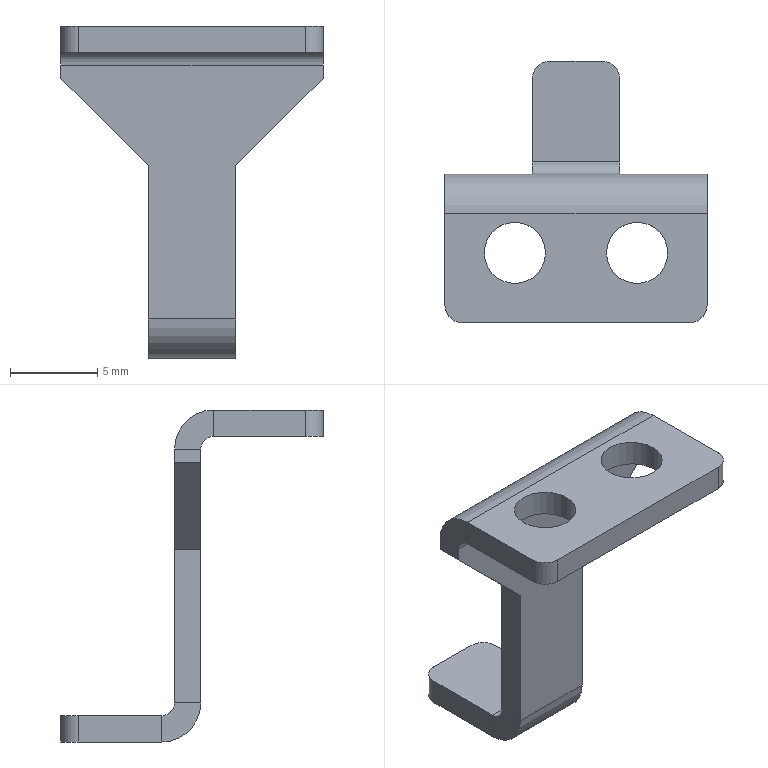Part | STEP file | 06-01-14 photoelectric sensor plate (Default) | 1 solid | 34 faces | box 15 x 15 x 19 mm | volume 381.957 mm3 | plane 22 | cylinder 12 | commonest cylinder face diameters 2 x4 3.5 x4 1.473 x2 4.473 x2
STEP:
#1=CARTESIAN_POINT('',(-5.25,0.5,0.));
#2=VERTEX_POINT('',#1);
#3=CARTESIAN_POINT('',(-1.75,0.5,0.));
#4=VERTEX_POINT('',#3);
#5=CARTESIAN_POINT('',(-3.5,0.5,0.));
#6=DIRECTION('',(0.,0.,1.));
#7=DIRECTION('',(1.,0.,0.));
#8=AXIS2_PLACEMENT_3D('',#5,#6,#7);
#9=CIRCLE('',#8,1.75);
#10=EDGE_CURVE('',#2,#4,#9,.T.);
#11=ORIENTED_EDGE('',*,*,#10,.T.);
#12=CARTESIAN_POINT('',(-1.75,0.5,-1.5));
#13=VERTEX_POINT('',#12);
#14=CARTESIAN_POINT('',(-1.75,0.5,3.5));
#15=DIRECTION('',(0.,0.,-1.));
#16=VECTOR('',#15,1000.);
#17=LINE('',#14,#16);
#18=EDGE_CURVE('',#4,#13,#17,.T.);
#19=ORIENTED_EDGE('',*,*,#18,.T.);
#20=CARTESIAN_POINT('',(-5.25,0.5,-1.5));
#21=VERTEX_POINT('',#20);
#22=CARTESIAN_POINT('',(-3.5,0.5,-1.5));
#23=DIRECTION('',(0.,0.,-1.));
#24=DIRECTION('',(-1.,0.,0.));
#25=AXIS2_PLACEMENT_3D('',#22,#23,#24);
#26=CIRCLE('',#25,1.75);
#27=EDGE_CURVE('',#13,#21,#26,.T.);
#28=ORIENTED_EDGE('',*,*,#27,.T.);
#29=CARTESIAN_POINT('',(-5.25,0.5,3.5));
#30=DIRECTION('',(0.,0.,-1.));
#31=VECTOR('',#30,1000.);
#32=LINE('',#29,#31);
#33=EDGE_CURVE('',#2,#21,#32,.T.);
#34=ORIENTED_EDGE('',*,*,#33,.F.);
#35=EDGE_LOOP('',(#11,#19,#28,#34));
#36=FACE_OUTER_BOUND('',#35,.T.);
#37=CARTESIAN_POINT('',(-3.5,0.5,3.5));
#38=DIRECTION('',(0.,0.,-1.));
#39=DIRECTION('',(-1.,0.,0.));
#40=AXIS2_PLACEMENT_3D('',#37,#38,#39);
#41=CYLINDRICAL_SURFACE('',#40,1.75);
#42=ADVANCED_FACE('',(#36),#41,.F.);
#43=CARTESIAN_POINT('',(1.75,0.5,0.));
#44=VERTEX_POINT('',#43);
#45=CARTESIAN_POINT('',(5.25,0.5,0.));
#46=VERTEX_POINT('',#45);
#47=CARTESIAN_POINT('',(3.5,0.5,0.));
#48=DIRECTION('',(0.,0.,1.));
#49=DIRECTION('',(1.,0.,0.));
#50=AXIS2_PLACEMENT_3D('',#47,#48,#49);
#51=CIRCLE('',#50,1.75);
#52=EDGE_CURVE('',#44,#46,#51,.T.);
#53=ORIENTED_EDGE('',*,*,#52,.T.);
#54=CARTESIAN_POINT('',(5.25,0.5,-1.5));
#55=VERTEX_POINT('',#54);
#56=CARTESIAN_POINT('',(5.25,0.5,3.5));
#57=DIRECTION('',(0.,0.,-1.));
#58=VECTOR('',#57,1000.);
#59=LINE('',#56,#58);
#60=EDGE_CURVE('',#46,#55,#59,.T.);
#61=ORIENTED_EDGE('',*,*,#60,.T.);
#62=CARTESIAN_POINT('',(1.75,0.5,-1.5));
#63=VERTEX_POINT('',#62);
#64=CARTESIAN_POINT('',(3.5,0.5,-1.5));
#65=DIRECTION('',(0.,0.,-1.));
#66=DIRECTION('',(-1.,0.,0.));
#67=AXIS2_PLACEMENT_3D('',#64,#65,#66);
#68=CIRCLE('',#67,1.75);
#69=EDGE_CURVE('',#55,#63,#68,.T.);
#70=ORIENTED_EDGE('',*,*,#69,.T.);
#71=CARTESIAN_POINT('',(1.75,0.5,3.5));
#72=DIRECTION('',(0.,0.,-1.));
#73=VECTOR('',#72,1000.);
#74=LINE('',#71,#73);
#75=EDGE_CURVE('',#44,#63,#74,.T.);
#76=ORIENTED_EDGE('',*,*,#75,.F.);
#77=EDGE_LOOP('',(#53,#61,#70,#76));
#78=FACE_OUTER_BOUND('',#77,.T.);
#79=CARTESIAN_POINT('',(3.5,0.5,3.5));
#80=DIRECTION('',(0.,0.,-1.));
#81=DIRECTION('',(-1.,0.,0.));
#82=AXIS2_PLACEMENT_3D('',#79,#80,#81);
#83=CYLINDRICAL_SURFACE('',#82,1.75);
#84=ADVANCED_FACE('',(#78),#83,.F.);
#85=CARTESIAN_POINT('',(7.5,5.,-3.));
#86=VERTEX_POINT('',#85);
#87=CARTESIAN_POINT('',(7.5,5.,-2.237));
#88=VERTEX_POINT('',#87);
#89=CARTESIAN_POINT('',(7.5,5.,-1.5));
#90=DIRECTION('',(0.,0.,1.));
#91=VECTOR('',#90,1000.);
#92=LINE('',#89,#91);
#93=EDGE_CURVE('',#86,#88,#92,.T.);
#94=ORIENTED_EDGE('',*,*,#93,.F.);
#95=CARTESIAN_POINT('',(2.5,5.,-8.));
#96=VERTEX_POINT('',#95);
#97=CARTESIAN_POINT('',(8.25,5.,-2.25));
#98=DIRECTION('',(0.7071,0.,0.7071));
#99=VECTOR('',#98,1000.);
#100=LINE('',#97,#99);
#101=EDGE_CURVE('',#96,#86,#100,.T.);
#102=ORIENTED_EDGE('',*,*,#101,.F.);
#103=CARTESIAN_POINT('',(2.5,5.,-16.763));
#104=VERTEX_POINT('',#103);
#105=CARTESIAN_POINT('',(2.5,5.,-1.5));
#106=DIRECTION('',(0.,0.,1.));
#107=VECTOR('',#106,1000.);
#108=LINE('',#105,#107);
#109=EDGE_CURVE('',#104,#96,#108,.T.);
#110=ORIENTED_EDGE('',*,*,#109,.F.);
#111=CARTESIAN_POINT('',(-2.5,5.,-16.763));
#112=VERTEX_POINT('',#111);
#113=CARTESIAN_POINT('',(-7.5,5.,-16.763));
#114=DIRECTION('',(1.,0.,0.));
#115=VECTOR('',#114,1000.);
#116=LINE('',#113,#115);
#117=EDGE_CURVE('',#112,#104,#116,.T.);
#118=ORIENTED_EDGE('',*,*,#117,.F.);
#119=CARTESIAN_POINT('',(-2.5,5.,-8.));
#120=VERTEX_POINT('',#119);
#121=CARTESIAN_POINT('',(-2.5,5.,-1.5));
#122=DIRECTION('',(0.,0.,-1.));
#123=VECTOR('',#122,1000.);
#124=LINE('',#121,#123);
#125=EDGE_CURVE('',#120,#112,#124,.T.);
#126=ORIENTED_EDGE('',*,*,#125,.F.);
#127=CARTESIAN_POINT('',(-7.5,5.,-3.));
#128=VERTEX_POINT('',#127);
#129=CARTESIAN_POINT('',(-0.75,5.,-9.75));
#130=DIRECTION('',(0.7071,0.,-0.7071));
#131=VECTOR('',#130,1000.);
#132=LINE('',#129,#131);
#133=EDGE_CURVE('',#128,#120,#132,.T.);
#134=ORIENTED_EDGE('',*,*,#133,.F.);
#135=CARTESIAN_POINT('',(-7.5,5.,-2.237));
#136=VERTEX_POINT('',#135);
#137=CARTESIAN_POINT('',(-7.5,5.,-17.5));
#138=DIRECTION('',(0.,0.,-1.));
#139=VECTOR('',#138,1000.);
#140=LINE('',#137,#139);
#141=EDGE_CURVE('',#136,#128,#140,.T.);
#142=ORIENTED_EDGE('',*,*,#141,.F.);
#143=CARTESIAN_POINT('',(7.5,5.,-2.237));
#144=DIRECTION('',(1.,0.,0.));
#145=VECTOR('',#144,1000.);
#146=LINE('',#143,#145);
#147=EDGE_CURVE('',#136,#88,#146,.T.);
#148=ORIENTED_EDGE('',*,*,#147,.T.);
#149=EDGE_LOOP('',(#94,#102,#110,#118,#126,#134,#142,#148));
#150=FACE_OUTER_BOUND('',#149,.T.);
#151=CARTESIAN_POINT('',(7.5,5.,-1.5));
#152=DIRECTION('',(0.,1.,0.));
#153=DIRECTION('',(0.,0.,1.));
#154=AXIS2_PLACEMENT_3D('',#151,#152,#153);
#155=PLANE('',#154);
#156=ADVANCED_FACE('',(#150),#155,.T.);
#157=CARTESIAN_POINT('',(2.5,3.5,-8.));
#158=VERTEX_POINT('',#157);
#159=CARTESIAN_POINT('',(7.5,3.5,-3.));
#160=VERTEX_POINT('',#159);
#161=CARTESIAN_POINT('',(8.25,3.5,-2.25));
#162=DIRECTION('',(0.7071,0.,0.7071));
#163=VECTOR('',#162,1000.);
#164=LINE('',#161,#163);
#165=EDGE_CURVE('',#158,#160,#164,.T.);
#166=ORIENTED_EDGE('',*,*,#165,.T.);
#167=CARTESIAN_POINT('',(7.5,3.5,-2.237));
#168=VERTEX_POINT('',#167);
#169=CARTESIAN_POINT('',(7.5,3.5,-1.5));
#170=DIRECTION('',(0.,0.,1.));
#171=VECTOR('',#170,1000.);
#172=LINE('',#169,#171);
#173=EDGE_CURVE('',#160,#168,#172,.T.);
#174=ORIENTED_EDGE('',*,*,#173,.T.);
#175=CARTESIAN_POINT('',(-7.5,3.5,-2.237));
#176=VERTEX_POINT('',#175);
#177=CARTESIAN_POINT('',(-7.5,3.5,-2.237));
#178=DIRECTION('',(1.,0.,0.));
#179=VECTOR('',#178,1000.);
#180=LINE('',#177,#179);
#181=EDGE_CURVE('',#176,#168,#180,.T.);
#182=ORIENTED_EDGE('',*,*,#181,.F.);
#183=CARTESIAN_POINT('',(-7.5,3.5,-3.));
#184=VERTEX_POINT('',#183);
#185=CARTESIAN_POINT('',(-7.5,3.5,-17.5));
#186=DIRECTION('',(0.,0.,-1.));
#187=VECTOR('',#186,1000.);
#188=LINE('',#185,#187);
#189=EDGE_CURVE('',#176,#184,#188,.T.);
#190=ORIENTED_EDGE('',*,*,#189,.T.);
#191=CARTESIAN_POINT('',(-2.5,3.5,-8.));
#192=VERTEX_POINT('',#191);
#193=CARTESIAN_POINT('',(-0.75,3.5,-9.75));
#194=DIRECTION('',(0.7071,0.,-0.7071));
#195=VECTOR('',#194,1000.);
#196=LINE('',#193,#195);
#197=EDGE_CURVE('',#184,#192,#196,.T.);
#198=ORIENTED_EDGE('',*,*,#197,.T.);
#199=CARTESIAN_POINT('',(-2.5,3.5,-16.763));
#200=VERTEX_POINT('',#199);
#201=CARTESIAN_POINT('',(-2.5,3.5,-1.5));
#202=DIRECTION('',(0.,0.,-1.));
#203=VECTOR('',#202,1000.);
#204=LINE('',#201,#203);
#205=EDGE_CURVE('',#192,#200,#204,.T.);
#206=ORIENTED_EDGE('',*,*,#205,.T.);
#207=CARTESIAN_POINT('',(2.5,3.5,-16.763));
#208=VERTEX_POINT('',#207);
#209=CARTESIAN_POINT('',(-7.5,3.5,-16.763));
#210=DIRECTION('',(1.,0.,0.));
#211=VECTOR('',#210,1000.);
#212=LINE('',#209,#211);
#213=EDGE_CURVE('',#200,#208,#212,.T.);
#214=ORIENTED_EDGE('',*,*,#213,.T.);
#215=CARTESIAN_POINT('',(2.5,3.5,-1.5));
#216=DIRECTION('',(0.,0.,1.));
#217=VECTOR('',#216,1000.);
#218=LINE('',#215,#217);
#219=EDGE_CURVE('',#208,#158,#218,.T.);
#220=ORIENTED_EDGE('',*,*,#219,.T.);
#221=EDGE_LOOP('',(#166,#174,#182,#190,#198,#206,#214,#220));
#222=FACE_OUTER_BOUND('',#221,.T.);
#223=CARTESIAN_POINT('',(7.5,3.5,-1.5));
#224=DIRECTION('',(0.,1.,0.));
#225=DIRECTION('',(0.,0.,1.));
#226=AXIS2_PLACEMENT_3D('',#223,#224,#225);
#227=PLANE('',#226);
#228=ADVANCED_FACE('',(#222),#227,.F.);
#229=CARTESIAN_POINT('',(2.5,5.737,-19.));
#230=VERTEX_POINT('',#229);
#231=CARTESIAN_POINT('',(-2.5,5.737,-19.));
#232=VERTEX_POINT('',#231);
#233=CARTESIAN_POINT('',(-7.5,5.737,-19.));
#234=DIRECTION('',(-1.,0.,0.));
#235=VECTOR('',#234,1000.);
#236=LINE('',#233,#235);
#237=EDGE_CURVE('',#230,#232,#236,.T.);
#238=ORIENTED_EDGE('',*,*,#237,.F.);
#239=CARTESIAN_POINT('',(2.5,5.737,-16.763));
#240=DIRECTION('',(1.,0.,0.));
#241=DIRECTION('',(0.,0.,1.));
#242=AXIS2_PLACEMENT_3D('',#239,#240,#241);
#243=CIRCLE('',#242,2.237);
#244=EDGE_CURVE('',#208,#230,#243,.T.);
#245=ORIENTED_EDGE('',*,*,#244,.F.);
#246=ORIENTED_EDGE('',*,*,#213,.F.);
#247=CARTESIAN_POINT('',(-2.5,5.737,-16.763));
#248=DIRECTION('',(-1.,0.,0.));
#249=DIRECTION('',(0.,0.,-1.));
#250=AXIS2_PLACEMENT_3D('',#247,#248,#249);
#251=CIRCLE('',#250,2.237);
#252=EDGE_CURVE('',#232,#200,#251,.T.);
#253=ORIENTED_EDGE('',*,*,#252,.F.);
#254=EDGE_LOOP('',(#238,#245,#246,#253));
#255=FACE_OUTER_BOUND('',#254,.T.);
#256=CARTESIAN_POINT('',(-7.5,5.737,-16.763));
#257=DIRECTION('',(-1.,0.,0.));
#258=DIRECTION('',(0.,0.,-1.));
#259=AXIS2_PLACEMENT_3D('',#256,#257,#258);
#260=CYLINDRICAL_SURFACE('',#259,2.237);
#261=ADVANCED_FACE('',(#255),#260,.T.);
#262=CARTESIAN_POINT('',(2.5,5.737,-17.5));
#263=VERTEX_POINT('',#262);
#264=CARTESIAN_POINT('',(2.5,5.737,-16.763));
#265=DIRECTION('',(1.,0.,0.));
#266=DIRECTION('',(0.,0.,1.));
#267=AXIS2_PLACEMENT_3D('',#264,#265,#266);
#268=CIRCLE('',#267,0.7366);
#269=EDGE_CURVE('',#104,#263,#268,.T.);
#270=ORIENTED_EDGE('',*,*,#269,.T.);
#271=CARTESIAN_POINT('',(-2.5,5.737,-17.5));
#272=VERTEX_POINT('',#271);
#273=CARTESIAN_POINT('',(7.5,5.737,-17.5));
#274=DIRECTION('',(-1.,0.,0.));
#275=VECTOR('',#274,1000.);
#276=LINE('',#273,#275);
#277=EDGE_CURVE('',#263,#272,#276,.T.);
#278=ORIENTED_EDGE('',*,*,#277,.T.);
#279=CARTESIAN_POINT('',(-2.5,5.737,-16.763));
#280=DIRECTION('',(-1.,0.,0.));
#281=DIRECTION('',(0.,0.,1.));
#282=AXIS2_PLACEMENT_3D('',#279,#280,#281);
#283=CIRCLE('',#282,0.7366);
#284=EDGE_CURVE('',#272,#112,#283,.T.);
#285=ORIENTED_EDGE('',*,*,#284,.T.);
#286=ORIENTED_EDGE('',*,*,#117,.T.);
#287=EDGE_LOOP('',(#270,#278,#285,#286));
#288=FACE_OUTER_BOUND('',#287,.T.);
#289=CARTESIAN_POINT('',(-7.5,5.737,-16.763));
#290=DIRECTION('',(-1.,0.,0.));
#291=DIRECTION('',(0.,0.,-1.));
#292=AXIS2_PLACEMENT_3D('',#289,#290,#291);
#293=CYLINDRICAL_SURFACE('',#292,0.7366);
#294=ADVANCED_FACE('',(#288),#293,.F.);
#295=CARTESIAN_POINT('',(1.5,11.5,-19.));
#296=VERTEX_POINT('',#295);
#297=CARTESIAN_POINT('',(-1.5,11.5,-19.));
#298=VERTEX_POINT('',#297);
#299=CARTESIAN_POINT('',(-7.5,11.5,-19.));
#300=DIRECTION('',(-1.,0.,0.));
#301=VECTOR('',#300,1000.);
#302=LINE('',#299,#301);
#303=EDGE_CURVE('',#296,#298,#302,.T.);
#304=ORIENTED_EDGE('',*,*,#303,.F.);
#305=CARTESIAN_POINT('',(2.5,10.5,-19.));
#306=VERTEX_POINT('',#305);
#307=CARTESIAN_POINT('',(1.5,10.5,-19.));
#308=DIRECTION('',(0.,0.,-1.));
#309=DIRECTION('',(-1.,0.,0.));
#310=AXIS2_PLACEMENT_3D('',#307,#308,#309);
#311=CIRCLE('',#310,1.);
#312=EDGE_CURVE('',#296,#306,#311,.T.);
#313=ORIENTED_EDGE('',*,*,#312,.T.);
#314=CARTESIAN_POINT('',(2.5,5.,-19.));
#315=DIRECTION('',(0.,1.,0.));
#316=VECTOR('',#315,1000.);
#317=LINE('',#314,#316);
#318=EDGE_CURVE('',#230,#306,#317,.T.);
#319=ORIENTED_EDGE('',*,*,#318,.F.);
#320=ORIENTED_EDGE('',*,*,#237,.T.);
#321=CARTESIAN_POINT('',(-2.5,10.5,-19.));
#322=VERTEX_POINT('',#321);
#323=CARTESIAN_POINT('',(-2.5,5.,-19.));
#324=DIRECTION('',(0.,-1.,0.));
#325=VECTOR('',#324,1000.);
#326=LINE('',#323,#325);
#327=EDGE_CURVE('',#322,#232,#326,.T.);
#328=ORIENTED_EDGE('',*,*,#327,.F.);
#329=CARTESIAN_POINT('',(-1.5,10.5,-19.));
#330=DIRECTION('',(0.,0.,-1.));
#331=DIRECTION('',(-1.,0.,0.));
#332=AXIS2_PLACEMENT_3D('',#329,#330,#331);
#333=CIRCLE('',#332,1.);
#334=EDGE_CURVE('',#322,#298,#333,.T.);
#335=ORIENTED_EDGE('',*,*,#334,.T.);
#336=EDGE_LOOP('',(#304,#313,#319,#320,#328,#335));
#337=FACE_OUTER_BOUND('',#336,.T.);
#338=CARTESIAN_POINT('',(-7.5,5.,-19.));
#339=DIRECTION('',(0.,0.,-1.));
#340=DIRECTION('',(-1.,0.,0.));
#341=AXIS2_PLACEMENT_3D('',#338,#339,#340);
#342=PLANE('',#341);
#343=ADVANCED_FACE('',(#337),#342,.T.);
#344=CARTESIAN_POINT('',(2.5,10.5,-17.5));
#345=VERTEX_POINT('',#344);
#346=CARTESIAN_POINT('',(2.5,5.,-17.5));
#347=DIRECTION('',(0.,1.,0.));
#348=VECTOR('',#347,1000.);
#349=LINE('',#346,#348);
#350=EDGE_CURVE('',#263,#345,#349,.T.);
#351=ORIENTED_EDGE('',*,*,#350,.T.);
#352=CARTESIAN_POINT('',(1.5,11.5,-17.5));
#353=VERTEX_POINT('',#352);
#354=CARTESIAN_POINT('',(1.5,10.5,-17.5));
#355=DIRECTION('',(0.,0.,1.));
#356=DIRECTION('',(-1.,0.,0.));
#357=AXIS2_PLACEMENT_3D('',#354,#355,#356);
#358=CIRCLE('',#357,1.);
#359=EDGE_CURVE('',#345,#353,#358,.T.);
#360=ORIENTED_EDGE('',*,*,#359,.T.);
#361=CARTESIAN_POINT('',(-1.5,11.5,-17.5));
#362=VERTEX_POINT('',#361);
#363=CARTESIAN_POINT('',(-7.5,11.5,-17.5));
#364=DIRECTION('',(-1.,0.,0.));
#365=VECTOR('',#364,1000.);
#366=LINE('',#363,#365);
#367=EDGE_CURVE('',#353,#362,#366,.T.);
#368=ORIENTED_EDGE('',*,*,#367,.T.);
#369=CARTESIAN_POINT('',(-2.5,10.5,-17.5));
#370=VERTEX_POINT('',#369);
#371=CARTESIAN_POINT('',(-1.5,10.5,-17.5));
#372=DIRECTION('',(0.,0.,1.));
#373=DIRECTION('',(-1.,0.,0.));
#374=AXIS2_PLACEMENT_3D('',#371,#372,#373);
#375=CIRCLE('',#374,1.);
#376=EDGE_CURVE('',#362,#370,#375,.T.);
#377=ORIENTED_EDGE('',*,*,#376,.T.);
#378=CARTESIAN_POINT('',(-2.5,5.,-17.5));
#379=DIRECTION('',(0.,-1.,0.));
#380=VECTOR('',#379,1000.);
#381=LINE('',#378,#380);
#382=EDGE_CURVE('',#370,#272,#381,.T.);
#383=ORIENTED_EDGE('',*,*,#382,.T.);
#384=ORIENTED_EDGE('',*,*,#277,.F.);
#385=EDGE_LOOP('',(#351,#360,#368,#377,#383,#384));
#386=FACE_OUTER_BOUND('',#385,.T.);
#387=CARTESIAN_POINT('',(-7.5,5.,-17.5));
#388=DIRECTION('',(0.,0.,-1.));
#389=DIRECTION('',(-1.,0.,0.));
#390=AXIS2_PLACEMENT_3D('',#387,#388,#389);
#391=PLANE('',#390);
#392=ADVANCED_FACE('',(#386),#391,.F.);
#393=ORIENTED_EDGE('',*,*,#367,.F.);
#394=CARTESIAN_POINT('',(1.5,11.5,-19.));
#395=DIRECTION('',(0.,0.,-1.));
#396=VECTOR('',#395,1000.);
#397=LINE('',#394,#396);
#398=EDGE_CURVE('',#353,#296,#397,.T.);
#399=ORIENTED_EDGE('',*,*,#398,.T.);
#400=ORIENTED_EDGE('',*,*,#303,.T.);
#401=CARTESIAN_POINT('',(-1.5,11.5,-19.));
#402=DIRECTION('',(0.,0.,1.));
#403=VECTOR('',#402,1000.);
#404=LINE('',#401,#403);
#405=EDGE_CURVE('',#298,#362,#404,.T.);
#406=ORIENTED_EDGE('',*,*,#405,.T.);
#407=EDGE_LOOP('',(#393,#399,#400,#406));
#408=FACE_OUTER_BOUND('',#407,.T.);
#409=CARTESIAN_POINT('',(-7.5,11.5,-19.));
#410=DIRECTION('',(0.,1.,0.));
#411=DIRECTION('',(0.,0.,1.));
#412=AXIS2_PLACEMENT_3D('',#409,#410,#411);
#413=PLANE('',#412);
#414=ADVANCED_FACE('',(#408),#413,.T.);
#415=ORIENTED_EDGE('',*,*,#173,.F.);
#416=CARTESIAN_POINT('',(7.5,5.,-3.));
#417=DIRECTION('',(0.,-1.,0.));
#418=VECTOR('',#417,1000.);
#419=LINE('',#416,#418);
#420=EDGE_CURVE('',#86,#160,#419,.T.);
#421=ORIENTED_EDGE('',*,*,#420,.F.);
#422=ORIENTED_EDGE('',*,*,#93,.T.);
#423=CARTESIAN_POINT('',(7.5,3.5,-2.237));
#424=DIRECTION('',(0.,1.,0.));
#425=VECTOR('',#424,1000.);
#426=LINE('',#423,#425);
#427=EDGE_CURVE('',#168,#88,#426,.T.);
#428=ORIENTED_EDGE('',*,*,#427,.F.);
#429=EDGE_LOOP('',(#415,#421,#422,#428));
#430=FACE_OUTER_BOUND('',#429,.T.);
#431=CARTESIAN_POINT('',(7.5,5.,-1.5));
#432=DIRECTION('',(1.,0.,0.));
#433=DIRECTION('',(0.,0.,-1.));
#434=AXIS2_PLACEMENT_3D('',#431,#432,#433);
#435=PLANE('',#434);
#436=ADVANCED_FACE('',(#430),#435,.T.);
#437=ORIENTED_EDGE('',*,*,#141,.T.);
#438=CARTESIAN_POINT('',(-7.5,5.,-3.));
#439=DIRECTION('',(0.,-1.,0.));
#440=VECTOR('',#439,1000.);
#441=LINE('',#438,#440);
#442=EDGE_CURVE('',#128,#184,#441,.T.);
#443=ORIENTED_EDGE('',*,*,#442,.T.);
#444=ORIENTED_EDGE('',*,*,#189,.F.);
#445=CARTESIAN_POINT('',(-7.5,3.5,-2.237));
#446=DIRECTION('',(0.,1.,0.));
#447=VECTOR('',#446,1000.);
#448=LINE('',#445,#447);
#449=EDGE_CURVE('',#176,#136,#448,.T.);
#450=ORIENTED_EDGE('',*,*,#449,.T.);
#451=EDGE_LOOP('',(#437,#443,#444,#450));
#452=FACE_OUTER_BOUND('',#451,.T.);
#453=CARTESIAN_POINT('',(-7.5,5.,-17.5));
#454=DIRECTION('',(-1.,0.,0.));
#455=DIRECTION('',(0.,0.,1.));
#456=AXIS2_PLACEMENT_3D('',#453,#454,#455);
#457=PLANE('',#456);
#458=ADVANCED_FACE('',(#452),#457,.T.);
#459=CARTESIAN_POINT('',(7.5,-2.5,0.));
#460=VERTEX_POINT('',#459);
#461=CARTESIAN_POINT('',(7.5,2.763,0.));
#462=VERTEX_POINT('',#461);
#463=CARTESIAN_POINT('',(7.5,3.5,0.));
#464=DIRECTION('',(0.,1.,0.));
#465=VECTOR('',#464,1000.);
#466=LINE('',#463,#465);
#467=EDGE_CURVE('',#460,#462,#466,.T.);
#468=ORIENTED_EDGE('',*,*,#467,.F.);
#469=CARTESIAN_POINT('',(7.5,-2.5,-1.5));
#470=VERTEX_POINT('',#469);
#471=CARTESIAN_POINT('',(7.5,-2.5,-1.5));
#472=DIRECTION('',(0.,0.,-1.));
#473=VECTOR('',#472,1000.);
#474=LINE('',#471,#473);
#475=EDGE_CURVE('',#460,#470,#474,.T.);
#476=ORIENTED_EDGE('',*,*,#475,.T.);
#477=CARTESIAN_POINT('',(7.5,2.763,-1.5));
#478=VERTEX_POINT('',#477);
#479=CARTESIAN_POINT('',(7.5,3.5,-1.5));
#480=DIRECTION('',(0.,1.,0.));
#481=VECTOR('',#480,1000.);
#482=LINE('',#479,#481);
#483=EDGE_CURVE('',#470,#478,#482,.T.);
#484=ORIENTED_EDGE('',*,*,#483,.T.);
#485=CARTESIAN_POINT('',(7.5,2.763,-1.5));
#486=DIRECTION('',(0.,0.,1.));
#487=VECTOR('',#486,1000.);
#488=LINE('',#485,#487);
#489=EDGE_CURVE('',#478,#462,#488,.T.);
#490=ORIENTED_EDGE('',*,*,#489,.T.);
#491=EDGE_LOOP('',(#468,#476,#484,#490));
#492=FACE_OUTER_BOUND('',#491,.T.);
#493=CARTESIAN_POINT('',(7.5,3.5,-1.5));
#494=DIRECTION('',(1.,0.,0.));
#495=DIRECTION('',(0.,1.,0.));
#496=AXIS2_PLACEMENT_3D('',#493,#494,#495);
#497=PLANE('',#496);
#498=ADVANCED_FACE('',(#492),#497,.T.);
#499=CARTESIAN_POINT('',(-3.5,0.5,-1.5));
#500=DIRECTION('',(0.,0.,-1.));
#501=DIRECTION('',(-1.,0.,0.));
#502=AXIS2_PLACEMENT_3D('',#499,#500,#501);
#503=CIRCLE('',#502,1.75);
#504=EDGE_CURVE('',#21,#13,#503,.T.);
#505=ORIENTED_EDGE('',*,*,#504,.F.);
#506=ORIENTED_EDGE('',*,*,#27,.F.);
#507=EDGE_LOOP('',(#505,#506));
#508=FACE_BOUND('',#507,.T.);
#509=CARTESIAN_POINT('',(3.5,0.5,-1.5));
#510=DIRECTION('',(0.,0.,-1.));
#511=DIRECTION('',(-1.,0.,0.));
#512=AXIS2_PLACEMENT_3D('',#509,#510,#511);
#513=CIRCLE('',#512,1.75);
#514=EDGE_CURVE('',#63,#55,#513,.T.);
#515=ORIENTED_EDGE('',*,*,#514,.F.);
#516=ORIENTED_EDGE('',*,*,#69,.F.);
#517=EDGE_LOOP('',(#515,#516));
#518=FACE_BOUND('',#517,.T.);
#519=ORIENTED_EDGE('',*,*,#483,.F.);
#520=CARTESIAN_POINT('',(6.5,-3.5,-1.5));
#521=VERTEX_POINT('',#520);
#522=CARTESIAN_POINT('',(6.5,-2.5,-1.5));
#523=DIRECTION('',(0.,0.,-1.));
#524=DIRECTION('',(1.,0.,0.));
#525=AXIS2_PLACEMENT_3D('',#522,#523,#524);
#526=CIRCLE('',#525,1.);
#527=EDGE_CURVE('',#470,#521,#526,.T.);
#528=ORIENTED_EDGE('',*,*,#527,.T.);
#529=CARTESIAN_POINT('',(-6.5,-3.5,-1.5));
#530=VERTEX_POINT('',#529);
#531=CARTESIAN_POINT('',(-7.5,-3.5,-1.5));
#532=DIRECTION('',(1.,0.,0.));
#533=VECTOR('',#532,1000.);
#534=LINE('',#531,#533);
#535=EDGE_CURVE('',#530,#521,#534,.T.);
#536=ORIENTED_EDGE('',*,*,#535,.F.);
#537=CARTESIAN_POINT('',(-7.5,-2.5,-1.5));
#538=VERTEX_POINT('',#537);
#539=CARTESIAN_POINT('',(-6.5,-2.5,-1.5));
#540=DIRECTION('',(0.,0.,-1.));
#541=DIRECTION('',(1.,0.,0.));
#542=AXIS2_PLACEMENT_3D('',#539,#540,#541);
#543=CIRCLE('',#542,1.);
#544=EDGE_CURVE('',#530,#538,#543,.T.);
#545=ORIENTED_EDGE('',*,*,#544,.T.);
#546=CARTESIAN_POINT('',(-7.5,2.763,-1.5));
#547=VERTEX_POINT('',#546);
#548=CARTESIAN_POINT('',(-7.5,3.5,-1.5));
#549=DIRECTION('',(0.,-1.,0.));
#550=VECTOR('',#549,1000.);
#551=LINE('',#548,#550);
#552=EDGE_CURVE('',#547,#538,#551,.T.);
#553=ORIENTED_EDGE('',*,*,#552,.F.);
#554=CARTESIAN_POINT('',(7.5,2.763,-1.5));
#555=DIRECTION('',(-1.,0.,0.));
#556=VECTOR('',#555,1000.);
#557=LINE('',#554,#556);
#558=EDGE_CURVE('',#478,#547,#557,.T.);
#559=ORIENTED_EDGE('',*,*,#558,.F.);
#560=EDGE_LOOP('',(#519,#528,#536,#545,#553,#559));
#561=FACE_OUTER_BOUND('',#560,.T.);
#562=CARTESIAN_POINT('',(7.5,-3.5,-1.5));
#563=DIRECTION('',(0.,0.,1.));
#564=DIRECTION('',(1.,0.,0.));
#565=AXIS2_PLACEMENT_3D('',#562,#563,#564);
#566=PLANE('',#565);
#567=ADVANCED_FACE('',(#508,#518,#561),#566,.F.);
#568=ORIENTED_EDGE('',*,*,#10,.F.);
#569=CARTESIAN_POINT('',(-3.5,0.5,0.));
#570=DIRECTION('',(0.,0.,1.));
#571=DIRECTION('',(1.,0.,0.));
#572=AXIS2_PLACEMENT_3D('',#569,#570,#571);
#573=CIRCLE('',#572,1.75);
#574=EDGE_CURVE('',#4,#2,#573,.T.);
#575=ORIENTED_EDGE('',*,*,#574,.F.);
#576=EDGE_LOOP('',(#568,#575));
#577=FACE_BOUND('',#576,.T.);
#578=ORIENTED_EDGE('',*,*,#52,.F.);
#579=CARTESIAN_POINT('',(3.5,0.5,0.));
#580=DIRECTION('',(0.,0.,1.));
#581=DIRECTION('',(1.,0.,0.));
#582=AXIS2_PLACEMENT_3D('',#579,#580,#581);
#583=CIRCLE('',#582,1.75);
#584=EDGE_CURVE('',#46,#44,#583,.T.);
#585=ORIENTED_EDGE('',*,*,#584,.F.);
#586=EDGE_LOOP('',(#578,#585));
#587=FACE_BOUND('',#586,.T.);
#588=CARTESIAN_POINT('',(-6.5,-3.5,0.));
#589=VERTEX_POINT('',#588);
#590=CARTESIAN_POINT('',(6.5,-3.5,0.));
#591=VERTEX_POINT('',#590);
#592=CARTESIAN_POINT('',(-7.5,-3.5,0.));
#593=DIRECTION('',(1.,0.,0.));
#594=VECTOR('',#593,1000.);
#595=LINE('',#592,#594);
#596=EDGE_CURVE('',#589,#591,#595,.T.);
#597=ORIENTED_EDGE('',*,*,#596,.T.);
#598=CARTESIAN_POINT('',(6.5,-2.5,0.));
#599=DIRECTION('',(0.,0.,1.));
#600=DIRECTION('',(1.,0.,0.));
#601=AXIS2_PLACEMENT_3D('',#598,#599,#600);
#602=CIRCLE('',#601,1.);
#603=EDGE_CURVE('',#591,#460,#602,.T.);
#604=ORIENTED_EDGE('',*,*,#603,.T.);
#605=ORIENTED_EDGE('',*,*,#467,.T.);
#606=CARTESIAN_POINT('',(-7.5,2.763,0.));
#607=VERTEX_POINT('',#606);
#608=CARTESIAN_POINT('',(7.5,2.763,0.));
#609=DIRECTION('',(-1.,0.,0.));
#610=VECTOR('',#609,1000.);
#611=LINE('',#608,#610);
#612=EDGE_CURVE('',#462,#607,#611,.T.);
#613=ORIENTED_EDGE('',*,*,#612,.T.);
#614=CARTESIAN_POINT('',(-7.5,-2.5,0.));
#615=VERTEX_POINT('',#614);
#616=CARTESIAN_POINT('',(-7.5,3.5,0.));
#617=DIRECTION('',(0.,-1.,0.));
#618=VECTOR('',#617,1000.);
#619=LINE('',#616,#618);
#620=EDGE_CURVE('',#607,#615,#619,.T.);
#621=ORIENTED_EDGE('',*,*,#620,.T.);
#622=CARTESIAN_POINT('',(-6.5,-2.5,0.));
#623=DIRECTION('',(0.,0.,1.));
#624=DIRECTION('',(1.,0.,0.));
#625=AXIS2_PLACEMENT_3D('',#622,#623,#624);
#626=CIRCLE('',#625,1.);
#627=EDGE_CURVE('',#615,#589,#626,.T.);
#628=ORIENTED_EDGE('',*,*,#627,.T.);
#629=EDGE_LOOP('',(#597,#604,#605,#613,#621,#628));
#630=FACE_OUTER_BOUND('',#629,.T.);
#631=CARTESIAN_POINT('',(7.5,-3.5,0.));
#632=DIRECTION('',(0.,0.,1.));
#633=DIRECTION('',(1.,0.,0.));
#634=AXIS2_PLACEMENT_3D('',#631,#632,#633);
#635=PLANE('',#634);
#636=ADVANCED_FACE('',(#577,#587,#630),#635,.T.);
#637=ORIENTED_EDGE('',*,*,#535,.T.);
#638=CARTESIAN_POINT('',(6.5,-3.5,-1.5));
#639=DIRECTION('',(0.,0.,1.));
#640=VECTOR('',#639,1000.);
#641=LINE('',#638,#640);
#642=EDGE_CURVE('',#521,#591,#641,.T.);
#643=ORIENTED_EDGE('',*,*,#642,.T.);
#644=ORIENTED_EDGE('',*,*,#596,.F.);
#645=CARTESIAN_POINT('',(-6.5,-3.5,-1.5));
#646=DIRECTION('',(0.,0.,-1.));
#647=VECTOR('',#646,1000.);
#648=LINE('',#645,#647);
#649=EDGE_CURVE('',#589,#530,#648,.T.);
#650=ORIENTED_EDGE('',*,*,#649,.T.);
#651=EDGE_LOOP('',(#637,#643,#644,#650));
#652=FACE_OUTER_BOUND('',#651,.T.);
#653=CARTESIAN_POINT('',(-7.5,-3.5,-1.5));
#654=DIRECTION('',(0.,-1.,0.));
#655=DIRECTION('',(0.,0.,-1.));
#656=AXIS2_PLACEMENT_3D('',#653,#654,#655);
#657=PLANE('',#656);
#658=ADVANCED_FACE('',(#652),#657,.T.);
#659=ORIENTED_EDGE('',*,*,#552,.T.);
#660=CARTESIAN_POINT('',(-7.5,-2.5,-1.5));
#661=DIRECTION('',(0.,0.,1.));
#662=VECTOR('',#661,1000.);
#663=LINE('',#660,#662);
#664=EDGE_CURVE('',#538,#615,#663,.T.);
#665=ORIENTED_EDGE('',*,*,#664,.T.);
#666=ORIENTED_EDGE('',*,*,#620,.F.);
#667=CARTESIAN_POINT('',(-7.5,2.763,-1.5));
#668=DIRECTION('',(0.,0.,1.));
#669=VECTOR('',#668,1000.);
#670=LINE('',#667,#669);
#671=EDGE_CURVE('',#547,#607,#670,.T.);
#672=ORIENTED_EDGE('',*,*,#671,.F.);
#673=EDGE_LOOP('',(#659,#665,#666,#672));
#674=FACE_OUTER_BOUND('',#673,.T.);
#675=CARTESIAN_POINT('',(-7.5,3.5,-1.5));
#676=DIRECTION('',(-1.,0.,0.));
#677=DIRECTION('',(0.,-1.,0.));
#678=AXIS2_PLACEMENT_3D('',#675,#676,#677);
#679=PLANE('',#678);
#680=ADVANCED_FACE('',(#674),#679,.T.);
#681=ORIENTED_EDGE('',*,*,#449,.F.);
#682=CARTESIAN_POINT('',(-7.5,2.763,-2.237));
#683=DIRECTION('',(-1.,0.,0.));
#684=DIRECTION('',(0.,0.,-1.));
#685=AXIS2_PLACEMENT_3D('',#682,#683,#684);
#686=CIRCLE('',#685,0.7366);
#687=EDGE_CURVE('',#547,#176,#686,.T.);
#688=ORIENTED_EDGE('',*,*,#687,.F.);
#689=ORIENTED_EDGE('',*,*,#671,.T.);
#690=CARTESIAN_POINT('',(-7.5,2.763,-2.237));
#691=DIRECTION('',(-1.,0.,0.));
#692=DIRECTION('',(0.,0.,-1.));
#693=AXIS2_PLACEMENT_3D('',#690,#691,#692);
#694=CIRCLE('',#693,2.237);
#695=EDGE_CURVE('',#607,#136,#694,.T.);
#696=ORIENTED_EDGE('',*,*,#695,.T.);
#697=EDGE_LOOP('',(#681,#688,#689,#696));
#698=FACE_OUTER_BOUND('',#697,.T.);
#699=CARTESIAN_POINT('',(-7.5,2.763,-2.237));
#700=DIRECTION('',(-1.,0.,0.));
#701=DIRECTION('',(0.,0.,1.));
#702=AXIS2_PLACEMENT_3D('',#699,#700,#701);
#703=PLANE('',#702);
#704=ADVANCED_FACE('',(#698),#703,.T.);
#705=CARTESIAN_POINT('',(7.5,2.763,-2.237));
#706=DIRECTION('',(1.,0.,0.));
#707=DIRECTION('',(0.,0.,-1.));
#708=AXIS2_PLACEMENT_3D('',#705,#706,#707);
#709=CIRCLE('',#708,0.7366);
#710=EDGE_CURVE('',#168,#478,#709,.T.);
#711=ORIENTED_EDGE('',*,*,#710,.F.);
#712=ORIENTED_EDGE('',*,*,#427,.T.);
#713=CARTESIAN_POINT('',(7.5,2.763,-2.237));
#714=DIRECTION('',(1.,0.,0.));
#715=DIRECTION('',(0.,0.,-1.));
#716=AXIS2_PLACEMENT_3D('',#713,#714,#715);
#717=CIRCLE('',#716,2.237);
#718=EDGE_CURVE('',#88,#462,#717,.T.);
#719=ORIENTED_EDGE('',*,*,#718,.T.);
#720=ORIENTED_EDGE('',*,*,#489,.F.);
#721=EDGE_LOOP('',(#711,#712,#719,#720));
#722=FACE_OUTER_BOUND('',#721,.T.);
#723=CARTESIAN_POINT('',(7.5,2.763,-2.237));
#724=DIRECTION('',(-1.,0.,0.));
#725=DIRECTION('',(0.,0.,1.));
#726=AXIS2_PLACEMENT_3D('',#723,#724,#725);
#727=PLANE('',#726);
#728=ADVANCED_FACE('',(#722),#727,.F.);
#729=ORIENTED_EDGE('',*,*,#612,.F.);
#730=ORIENTED_EDGE('',*,*,#718,.F.);
#731=ORIENTED_EDGE('',*,*,#147,.F.);
#732=ORIENTED_EDGE('',*,*,#695,.F.);
#733=EDGE_LOOP('',(#729,#730,#731,#732));
#734=FACE_OUTER_BOUND('',#733,.T.);
#735=CARTESIAN_POINT('',(7.5,2.763,-2.237));
#736=DIRECTION('',(1.,0.,0.));
#737=DIRECTION('',(0.,1.,0.));
#738=AXIS2_PLACEMENT_3D('',#735,#736,#737);
#739=CYLINDRICAL_SURFACE('',#738,2.237);
#740=ADVANCED_FACE('',(#734),#739,.T.);
#741=ORIENTED_EDGE('',*,*,#558,.T.);
#742=ORIENTED_EDGE('',*,*,#687,.T.);
#743=ORIENTED_EDGE('',*,*,#181,.T.);
#744=ORIENTED_EDGE('',*,*,#710,.T.);
#745=EDGE_LOOP('',(#741,#742,#743,#744));
#746=FACE_OUTER_BOUND('',#745,.T.);
#747=CARTESIAN_POINT('',(7.5,2.763,-2.237));
#748=DIRECTION('',(1.,0.,0.));
#749=DIRECTION('',(0.,1.,0.));
#750=AXIS2_PLACEMENT_3D('',#747,#748,#749);
#751=CYLINDRICAL_SURFACE('',#750,0.7366);
#752=ADVANCED_FACE('',(#746),#751,.F.);
#753=ORIENTED_EDGE('',*,*,#60,.F.);
#754=ORIENTED_EDGE('',*,*,#584,.T.);
#755=ORIENTED_EDGE('',*,*,#75,.T.);
#756=ORIENTED_EDGE('',*,*,#514,.T.);
#757=EDGE_LOOP('',(#753,#754,#755,#756));
#758=FACE_OUTER_BOUND('',#757,.T.);
#759=CARTESIAN_POINT('',(3.5,0.5,3.5));
#760=DIRECTION('',(0.,0.,-1.));
#761=DIRECTION('',(-1.,0.,0.));
#762=AXIS2_PLACEMENT_3D('',#759,#760,#761);
#763=CYLINDRICAL_SURFACE('',#762,1.75);
#764=ADVANCED_FACE('',(#758),#763,.F.);
#765=ORIENTED_EDGE('',*,*,#18,.F.);
#766=ORIENTED_EDGE('',*,*,#574,.T.);
#767=ORIENTED_EDGE('',*,*,#33,.T.);
#768=ORIENTED_EDGE('',*,*,#504,.T.);
#769=EDGE_LOOP('',(#765,#766,#767,#768));
#770=FACE_OUTER_BOUND('',#769,.T.);
#771=CARTESIAN_POINT('',(-3.5,0.5,3.5));
#772=DIRECTION('',(0.,0.,-1.));
#773=DIRECTION('',(-1.,0.,0.));
#774=AXIS2_PLACEMENT_3D('',#771,#772,#773);
#775=CYLINDRICAL_SURFACE('',#774,1.75);
#776=ADVANCED_FACE('',(#770),#775,.F.);
#777=ORIENTED_EDGE('',*,*,#442,.F.);
#778=ORIENTED_EDGE('',*,*,#133,.T.);
#779=CARTESIAN_POINT('',(-2.5,5.,-8.));
#780=DIRECTION('',(0.,-1.,0.));
#781=VECTOR('',#780,1000.);
#782=LINE('',#779,#781);
#783=EDGE_CURVE('',#120,#192,#782,.T.);
#784=ORIENTED_EDGE('',*,*,#783,.T.);
#785=ORIENTED_EDGE('',*,*,#197,.F.);
#786=EDGE_LOOP('',(#777,#778,#784,#785));
#787=FACE_OUTER_BOUND('',#786,.T.);
#788=CARTESIAN_POINT('',(-0.75,5.,-9.75));
#789=DIRECTION('',(0.7071,0.,0.7071));
#790=DIRECTION('',(0.7071,0.,-0.7071));
#791=AXIS2_PLACEMENT_3D('',#788,#789,#790);
#792=PLANE('',#791);
#793=ADVANCED_FACE('',(#787),#792,.F.);
#794=ORIENTED_EDGE('',*,*,#125,.T.);
#795=CARTESIAN_POINT('',(-2.5,5.,-16.763));
#796=DIRECTION('',(0.,-1.,0.));
#797=VECTOR('',#796,1000.);
#798=LINE('',#795,#797);
#799=EDGE_CURVE('',#112,#200,#798,.T.);
#800=ORIENTED_EDGE('',*,*,#799,.T.);
#801=ORIENTED_EDGE('',*,*,#205,.F.);
#802=ORIENTED_EDGE('',*,*,#783,.F.);
#803=EDGE_LOOP('',(#794,#800,#801,#802));
#804=FACE_OUTER_BOUND('',#803,.T.);
#805=CARTESIAN_POINT('',(-2.5,5.,-1.5));
#806=DIRECTION('',(1.,0.,0.));
#807=DIRECTION('',(0.,0.,-1.));
#808=AXIS2_PLACEMENT_3D('',#805,#806,#807);
#809=PLANE('',#808);
#810=ADVANCED_FACE('',(#804),#809,.F.);
#811=ORIENTED_EDGE('',*,*,#382,.F.);
#812=CARTESIAN_POINT('',(-2.5,10.5,-19.));
#813=DIRECTION('',(0.,0.,-1.));
#814=VECTOR('',#813,1000.);
#815=LINE('',#812,#814);
#816=EDGE_CURVE('',#370,#322,#815,.T.);
#817=ORIENTED_EDGE('',*,*,#816,.T.);
#818=ORIENTED_EDGE('',*,*,#327,.T.);
#819=CARTESIAN_POINT('',(-2.5,5.737,-19.));
#820=DIRECTION('',(0.,0.,1.));
#821=VECTOR('',#820,1000.);
#822=LINE('',#819,#821);
#823=EDGE_CURVE('',#232,#272,#822,.T.);
#824=ORIENTED_EDGE('',*,*,#823,.T.);
#825=EDGE_LOOP('',(#811,#817,#818,#824));
#826=FACE_OUTER_BOUND('',#825,.T.);
#827=CARTESIAN_POINT('',(-2.5,5.,-19.));
#828=DIRECTION('',(1.,0.,0.));
#829=DIRECTION('',(0.,-1.,0.));
#830=AXIS2_PLACEMENT_3D('',#827,#828,#829);
#831=PLANE('',#830);
#832=ADVANCED_FACE('',(#826),#831,.F.);
#833=ORIENTED_EDGE('',*,*,#252,.T.);
#834=ORIENTED_EDGE('',*,*,#799,.F.);
#835=ORIENTED_EDGE('',*,*,#284,.F.);
#836=ORIENTED_EDGE('',*,*,#823,.F.);
#837=EDGE_LOOP('',(#833,#834,#835,#836));
#838=FACE_OUTER_BOUND('',#837,.T.);
#839=CARTESIAN_POINT('',(-2.5,5.737,-16.763));
#840=DIRECTION('',(-1.,0.,0.));
#841=DIRECTION('',(0.,0.,1.));
#842=AXIS2_PLACEMENT_3D('',#839,#840,#841);
#843=PLANE('',#842);
#844=ADVANCED_FACE('',(#838),#843,.T.);
#845=CARTESIAN_POINT('',(2.5,5.,-8.));
#846=DIRECTION('',(0.,-1.,0.));
#847=VECTOR('',#846,1000.);
#848=LINE('',#845,#847);
#849=EDGE_CURVE('',#96,#158,#848,.T.);
#850=ORIENTED_EDGE('',*,*,#849,.F.);
#851=ORIENTED_EDGE('',*,*,#101,.T.);
#852=ORIENTED_EDGE('',*,*,#420,.T.);
#853=ORIENTED_EDGE('',*,*,#165,.F.);
#854=EDGE_LOOP('',(#850,#851,#852,#853));
#855=FACE_OUTER_BOUND('',#854,.T.);
#856=CARTESIAN_POINT('',(8.25,5.,-2.25));
#857=DIRECTION('',(-0.7071,0.,0.7071));
#858=DIRECTION('',(0.7071,0.,0.7071));
#859=AXIS2_PLACEMENT_3D('',#856,#857,#858);
#860=PLANE('',#859);
#861=ADVANCED_FACE('',(#855),#860,.F.);
#862=ORIENTED_EDGE('',*,*,#109,.T.);
#863=ORIENTED_EDGE('',*,*,#849,.T.);
#864=ORIENTED_EDGE('',*,*,#219,.F.);
#865=CARTESIAN_POINT('',(2.5,5.,-16.763));
#866=DIRECTION('',(0.,-1.,0.));
#867=VECTOR('',#866,1000.);
#868=LINE('',#865,#867);
#869=EDGE_CURVE('',#104,#208,#868,.T.);
#870=ORIENTED_EDGE('',*,*,#869,.F.);
#871=EDGE_LOOP('',(#862,#863,#864,#870));
#872=FACE_OUTER_BOUND('',#871,.T.);
#873=CARTESIAN_POINT('',(2.5,5.,-1.5));
#874=DIRECTION('',(-1.,0.,0.));
#875=DIRECTION('',(0.,0.,1.));
#876=AXIS2_PLACEMENT_3D('',#873,#874,#875);
#877=PLANE('',#876);
#878=ADVANCED_FACE('',(#872),#877,.F.);
#879=ORIENTED_EDGE('',*,*,#318,.T.);
#880=CARTESIAN_POINT('',(2.5,10.5,-17.5));
#881=DIRECTION('',(0.,0.,1.));
#882=VECTOR('',#881,1000.);
#883=LINE('',#880,#882);
#884=EDGE_CURVE('',#306,#345,#883,.T.);
#885=ORIENTED_EDGE('',*,*,#884,.T.);
#886=ORIENTED_EDGE('',*,*,#350,.F.);
#887=CARTESIAN_POINT('',(2.5,5.737,-17.5));
#888=DIRECTION('',(0.,0.,-1.));
#889=VECTOR('',#888,1000.);
#890=LINE('',#887,#889);
#891=EDGE_CURVE('',#263,#230,#890,.T.);
#892=ORIENTED_EDGE('',*,*,#891,.T.);
#893=EDGE_LOOP('',(#879,#885,#886,#892));
#894=FACE_OUTER_BOUND('',#893,.T.);
#895=CARTESIAN_POINT('',(2.5,5.,-17.5));
#896=DIRECTION('',(-1.,0.,0.));
#897=DIRECTION('',(0.,1.,0.));
#898=AXIS2_PLACEMENT_3D('',#895,#896,#897);
#899=PLANE('',#898);
#900=ADVANCED_FACE('',(#894),#899,.F.);
#901=ORIENTED_EDGE('',*,*,#891,.F.);
#902=ORIENTED_EDGE('',*,*,#269,.F.);
#903=ORIENTED_EDGE('',*,*,#869,.T.);
#904=ORIENTED_EDGE('',*,*,#244,.T.);
#905=EDGE_LOOP('',(#901,#902,#903,#904));
#906=FACE_OUTER_BOUND('',#905,.T.);
#907=CARTESIAN_POINT('',(2.5,5.737,-16.763));
#908=DIRECTION('',(1.,0.,0.));
#909=DIRECTION('',(0.,0.,-1.));
#910=AXIS2_PLACEMENT_3D('',#907,#908,#909);
#911=PLANE('',#910);
#912=ADVANCED_FACE('',(#906),#911,.T.);
#913=ORIENTED_EDGE('',*,*,#359,.F.);
#914=ORIENTED_EDGE('',*,*,#884,.F.);
#915=ORIENTED_EDGE('',*,*,#312,.F.);
#916=ORIENTED_EDGE('',*,*,#398,.F.);
#917=EDGE_LOOP('',(#913,#914,#915,#916));
#918=FACE_OUTER_BOUND('',#917,.T.);
#919=CARTESIAN_POINT('',(1.5,10.5,-19.));
#920=DIRECTION('',(0.,0.,1.));
#921=DIRECTION('',(1.,0.,0.));
#922=AXIS2_PLACEMENT_3D('',#919,#920,#921);
#923=CYLINDRICAL_SURFACE('',#922,1.);
#924=ADVANCED_FACE('',(#918),#923,.T.);
#925=ORIENTED_EDGE('',*,*,#334,.F.);
#926=ORIENTED_EDGE('',*,*,#816,.F.);
#927=ORIENTED_EDGE('',*,*,#376,.F.);
#928=ORIENTED_EDGE('',*,*,#405,.F.);
#929=EDGE_LOOP('',(#925,#926,#927,#928));
#930=FACE_OUTER_BOUND('',#929,.T.);
#931=CARTESIAN_POINT('',(-1.5,10.5,-19.));
#932=DIRECTION('',(0.,0.,-1.));
#933=DIRECTION('',(-1.,0.,0.));
#934=AXIS2_PLACEMENT_3D('',#931,#932,#933);
#935=CYLINDRICAL_SURFACE('',#934,1.);
#936=ADVANCED_FACE('',(#930),#935,.T.);
#937=ORIENTED_EDGE('',*,*,#527,.F.);
#938=ORIENTED_EDGE('',*,*,#475,.F.);
#939=ORIENTED_EDGE('',*,*,#603,.F.);
#940=ORIENTED_EDGE('',*,*,#642,.F.);
#941=EDGE_LOOP('',(#937,#938,#939,#940));
#942=FACE_OUTER_BOUND('',#941,.T.);
#943=CARTESIAN_POINT('',(6.5,-2.5,-1.5));
#944=DIRECTION('',(0.,0.,1.));
#945=DIRECTION('',(1.,0.,0.));
#946=AXIS2_PLACEMENT_3D('',#943,#944,#945);
#947=CYLINDRICAL_SURFACE('',#946,1.);
#948=ADVANCED_FACE('',(#942),#947,.T.);
#949=ORIENTED_EDGE('',*,*,#544,.F.);
#950=ORIENTED_EDGE('',*,*,#649,.F.);
#951=ORIENTED_EDGE('',*,*,#627,.F.);
#952=ORIENTED_EDGE('',*,*,#664,.F.);
#953=EDGE_LOOP('',(#949,#950,#951,#952));
#954=FACE_OUTER_BOUND('',#953,.T.);
#955=CARTESIAN_POINT('',(-6.5,-2.5,-1.5));
#956=DIRECTION('',(0.,0.,1.));
#957=DIRECTION('',(1.,0.,0.));
#958=AXIS2_PLACEMENT_3D('',#955,#956,#957);
#959=CYLINDRICAL_SURFACE('',#958,1.);
#960=ADVANCED_FACE('',(#954),#959,.T.);
#961=CLOSED_SHELL('',(#42,#84,#156,#228,#261,#294,#343,#392,#414,#436,#458,#498,#567,#636,#658,#680,#704,#728,#740,#752,#764,#776,#793,#810,#832,#844,#861,#878,#900,#912,#924,#936,#948,#960));
#962=MANIFOLD_SOLID_BREP('',#961);
#963=CARTESIAN_POINT('',(0.,0.,0.));
#964=DIRECTION('',(0.,0.,1.));
#965=DIRECTION('',(1.,0.,0.));
#966=AXIS2_PLACEMENT_3D('',#963,#964,#965);
#967=(LENGTH_UNIT()NAMED_UNIT(*)SI_UNIT(.MILLI.,.METRE.));
#968=UNCERTAINTY_MEASURE_WITH_UNIT(LENGTH_MEASURE(0.00001),#967,'','');
#969=(NAMED_UNIT(*)PLANE_ANGLE_UNIT()SI_UNIT($,.RADIAN.));
#970=(NAMED_UNIT(*)SI_UNIT($,.STERADIAN.)SOLID_ANGLE_UNIT());
#971=(GEOMETRIC_REPRESENTATION_CONTEXT(3)GLOBAL_UNCERTAINTY_ASSIGNED_CONTEXT((#968))GLOBAL_UNIT_ASSIGNED_CONTEXT((#967,#969,#970))REPRESENTATION_CONTEXT('',''));
#972=ADVANCED_BREP_SHAPE_REPRESENTATION('',(#962,#966),#971);